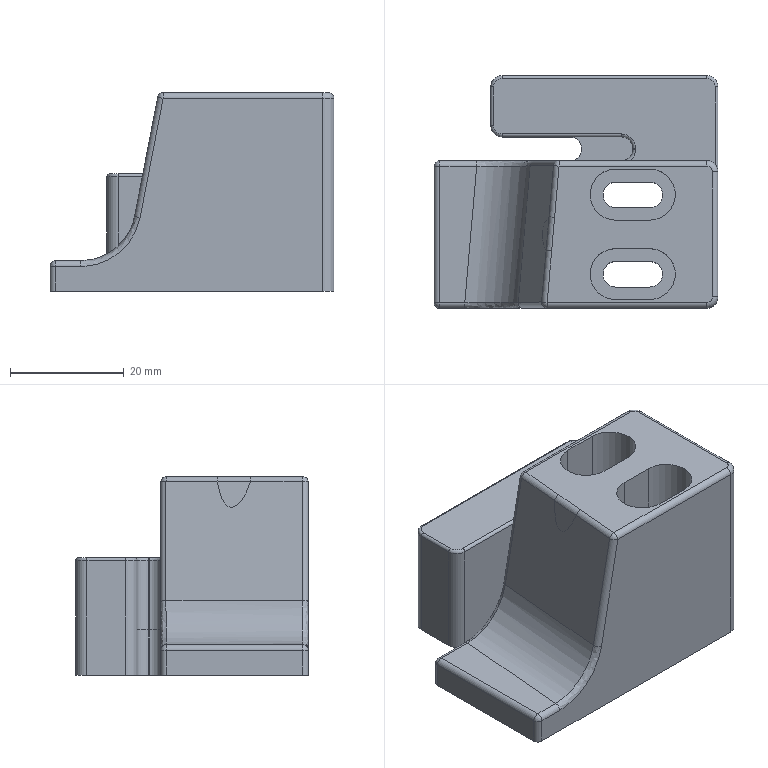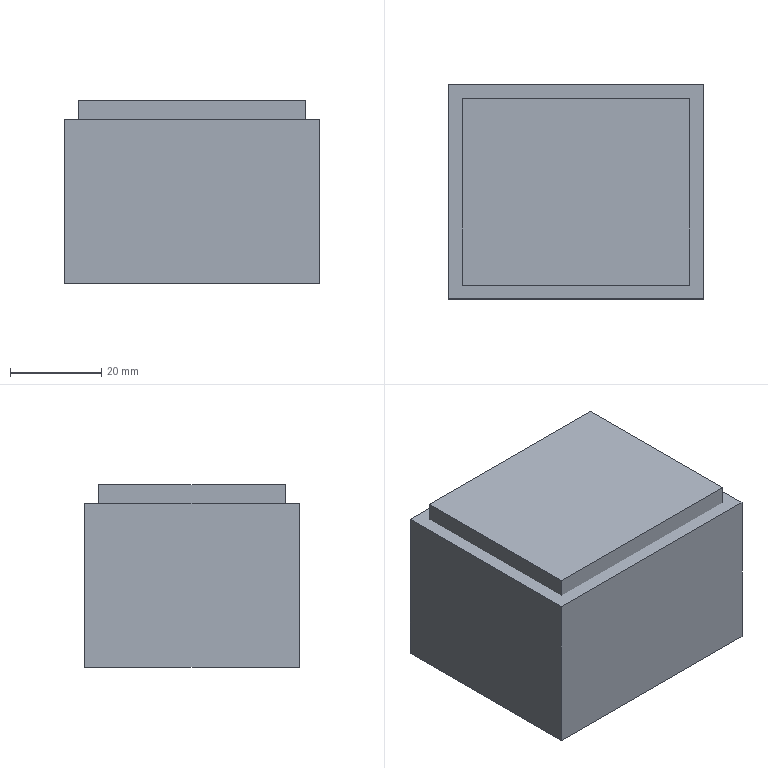CAM job | NX | 3-axis milling | part box 50 x 41 x 35 mm | stock box 56 x 47 x 40 mm
Tools:
number,name,description,diameter,corner_radius,flute_length,length,flutes
1,D63,Milling Tool-5 Parameters,63.0,0.0,50.0,75.0,2
9,D10,Milling Tool-5 Parameters,10.0,0.0,50.0,75.0,2
10,D10JING,Milling Tool-5 Parameters,10.0,0.0,50.0,75.0,2
4,D4,Milling Tool-5 Parameters,4.0,0.0,50.0,75.0,2
6,D6,Milling Tool-5 Parameters,6.0,0.0,50.0,75.0,2
8,D6R0.5,Milling Tool-5 Parameters,6.0,0.5,50.0,75.0,2
5,D4R0.5,Milling Tool-5 Parameters,4.0,0.5,50.0,75.0,2
2,D4A45,Milling Tool-5 Parameters,4.0,0.0,2.0,2.0,2
Operations:
program,operation,operation_type,tool,method,geometry_group,spindle_rpm,surface_speed,feed_per_tooth,feed_cut,feed_plunge,cut_length_mm,path_length_mm,cut_time_min,machine_time_min
1,FLOOR_WALL,VolumeBased25DMillingOperation,D63,METHOD,A,6500.0,1286.0,0.0962,1250.0,100.0,131.0,185.0,0.1048,0.1102
1,CAVITY_MILL,CavityMilling,D10,METHOD,A,9500.0,298.0,0.1579,3000.0,1000.0,19748.041,20251.117,6.816,6.867
1,ZLEVEL_PROFILE_COPY_COPY,ZLevelMilling,D10JING,METHOD,A,9500.0,119.0,0.0632,1200.0,1000.0,432.659,655.039,0.3619,0.3842
1,FLOOR_WALL_1,VolumeBased25DMillingOperation,D10JING,METHOD,A,9500.0,119.0,0.0526,1000.0,100.0,448.312,972.552,0.4483,0.5007
1,ZLEVEL_PROFILE_COPY_COPY_1_COPY,ZLevelMilling,D6,METHOD,A,9500.0,179.0,0.1158,2200.0,1000.0,1765.711,1934.971,0.8443,0.8612
1,ZLEVEL_PROFILE_COPY_COPY_COPY,ZLevelMilling,D6,METHOD,A,9500.0,119.0,0.0632,1200.0,1000.0,111.407,475.942,0.0949,0.1314
1,CAVITY_MILL_COPY,CavityMilling,D6,METHOD,A,9500.0,119.0,0.1053,2000.0,1000.0,406.362,788.754,0.2473,0.2855
1,CAVITY_MILL_COPY_COPY,CavityMilling,D4,METHOD,A,9500.0,119.0,0.0737,1400.0,1000.0,1748.119,1932.962,1.266,1.284
1,ZLEVEL_PROFILE_COPY,ZLevelMilling,D6R0.5,METHOD,A,9500.0,179.0,0.1579,3000.0,1000.0,2896.422,2954.934,0.9676,0.9734
1,ZLEVEL_PROFILE_COPY_COPY_1,ZLevelMilling,D6R0.5,METHOD,A,9500.0,179.0,0.1579,3000.0,1000.0,12561.031,20312.385,4.27,5.045
1,ZLEVEL_PROFILE_COPY_COPY_1_COPY_1,ZLevelMilling,D6R0.5,METHOD,A,9500.0,179.0,0.1579,3000.0,1000.0,1211.399,1448.373,0.407,0.4307
1,ZLEVEL_PROFILE_COPY_COPY_1_COPY_1_COPY,ZLevelMilling,D4R0.5,METHOD,A,9500.0,179.0,0.1579,3000.0,1000.0,1445.349,1531.949,0.4828,0.4915
1,ZLEVEL_PROFILE_1_COPY_1_COPY_COPY,ZLevelMilling,D4A45,METHOD,A,9500.0,179.0,0.0526,1000.0,100.0,77.194,211.373,0.0772,0.0906
2,FLOOR_WALL_COPY,VolumeBased25DMillingOperation,D63,METHOD,B,6500.0,1286.0,0.0962,1250.0,100.0,625.0,1351.001,0.5,0.5726
2,ZLEVEL_PROFILE_COPY_COPY_1_COPY_COPY,ZLevelMilling,D4,METHOD,B,9500.0,119.0,0.0632,1200.0,1000.0,1124.561,1282.372,0.9492,0.965
2,ZLEVEL_PROFILE_1_COPY_1_COPY_COPY_COPY,ZLevelMilling,D4A45,METHOD,B,9500.0,179.0,0.0526,1000.0,100.0,266.745,503.393,0.2667,0.2904